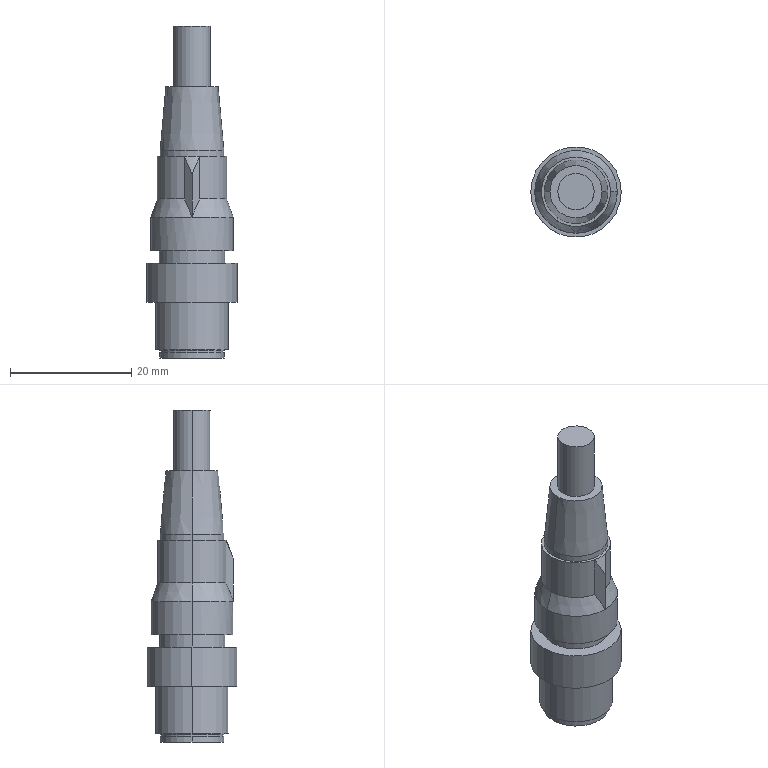Part | STEP file | E2EW-X7D118-M1TGJ0.3M-Part-4 | 1 solid | 49 faces | box 14.9 x 14.9 x 54.7 mm | volume 4876 mm3 | cylinder 26 | plane 17 | cone 6 | commonest cylinder face diameters 10.6 x4 11.4 x3 1 x2 6 x2 8.3 x2 10.2 x2